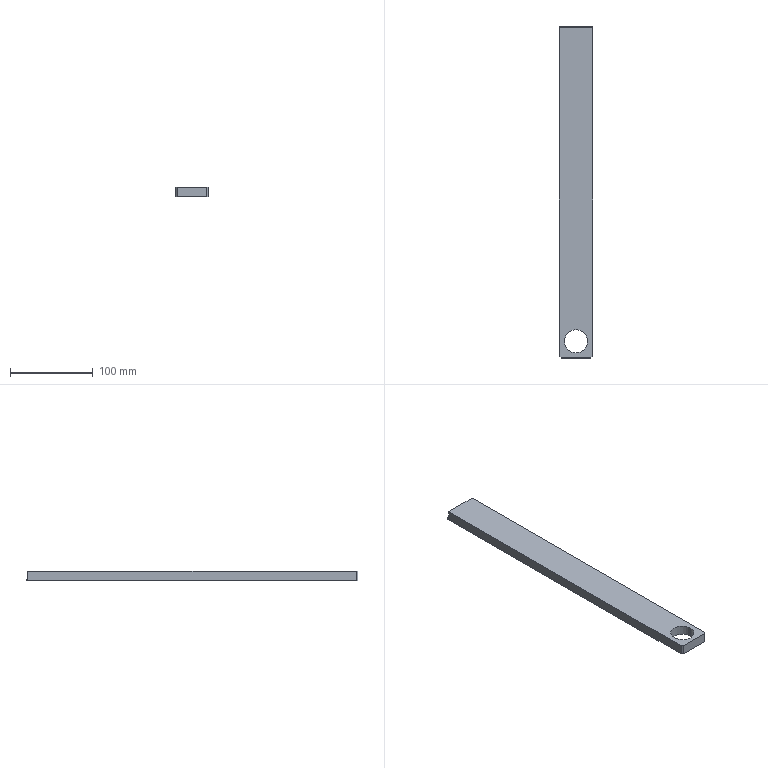Part | STEP file | 11-FG-B05811 | 1 solid | 28 faces | box 40 x 400 x 12 mm | volume 182663 mm3 | cylinder 10 | plane 10 | cone 8 | commonest cylinder face diameters 5 x8 28 x2
STEP:
#1=CARTESIAN_POINT('',(15.,386.,4.5));
#2=VERTEX_POINT('',#1);
#3=CARTESIAN_POINT('',(15.,386.,9.5));
#4=VERTEX_POINT('',#3);
#5=CARTESIAN_POINT('',(15.,386.,7.));
#6=DIRECTION('',(0.,1.,0.));
#7=DIRECTION('',(0.,0.,1.));
#8=AXIS2_PLACEMENT_3D('',#5,#6,#7);
#9=CIRCLE('',#8,2.5);
#10=EDGE_CURVE('',#2,#4,#9,.T.);
#11=ORIENTED_EDGE('',*,*,#10,.F.);
#12=CARTESIAN_POINT('',(15.,398.,4.5));
#13=VERTEX_POINT('',#12);
#14=CARTESIAN_POINT('',(15.,398.,4.5));
#15=DIRECTION('',(0.,1.,0.));
#16=VECTOR('',#15,1000.);
#17=LINE('',#14,#16);
#18=EDGE_CURVE('',#2,#13,#17,.T.);
#19=ORIENTED_EDGE('',*,*,#18,.T.);
#20=CARTESIAN_POINT('',(15.,398.,9.5));
#21=VERTEX_POINT('',#20);
#22=CARTESIAN_POINT('',(15.,398.,7.));
#23=DIRECTION('',(0.,1.,0.));
#24=DIRECTION('',(0.,0.,1.));
#25=AXIS2_PLACEMENT_3D('',#22,#23,#24);
#26=CIRCLE('',#25,2.5);
#27=EDGE_CURVE('',#13,#21,#26,.T.);
#28=ORIENTED_EDGE('',*,*,#27,.T.);
#29=CARTESIAN_POINT('',(15.,398.,9.5));
#30=DIRECTION('',(0.,1.,0.));
#31=VECTOR('',#30,1000.);
#32=LINE('',#29,#31);
#33=EDGE_CURVE('',#4,#21,#32,.T.);
#34=ORIENTED_EDGE('',*,*,#33,.F.);
#35=EDGE_LOOP('',(#11,#19,#28,#34));
#36=FACE_OUTER_BOUND('',#35,.T.);
#37=CARTESIAN_POINT('',(15.,398.,7.));
#38=DIRECTION('',(0.,1.,0.));
#39=DIRECTION('',(0.,0.,1.));
#40=AXIS2_PLACEMENT_3D('',#37,#38,#39);
#41=CYLINDRICAL_SURFACE('',#40,2.5);
#42=ADVANCED_FACE('',(#36),#41,.F.);
#43=CARTESIAN_POINT('',(15.,384.498,7.));
#44=VERTEX_POINT('',#43);
#45=CARTESIAN_POINT('',(15.,386.,9.5));
#46=DIRECTION('',(0.,0.515,0.8572));
#47=VECTOR('',#46,1000.);
#48=LINE('',#45,#47);
#49=EDGE_CURVE('',#44,#4,#48,.T.);
#50=ORIENTED_EDGE('',*,*,#49,.F.);
#51=CARTESIAN_POINT('',(15.,386.,4.5));
#52=DIRECTION('',(0.,0.515,-0.8572));
#53=VECTOR('',#52,1000.);
#54=LINE('',#51,#53);
#55=EDGE_CURVE('',#44,#2,#54,.T.);
#56=ORIENTED_EDGE('',*,*,#55,.T.);
#57=ORIENTED_EDGE('',*,*,#10,.T.);
#58=EDGE_LOOP('',(#50,#56,#57));
#59=FACE_OUTER_BOUND('',#58,.T.);
#60=CARTESIAN_POINT('',(15.,386.,7.));
#61=DIRECTION('',(0.,1.,0.));
#62=DIRECTION('',(0.,0.,1.));
#63=AXIS2_PLACEMENT_3D('',#60,#61,#62);
#64=CONICAL_SURFACE('',#63,2.5,1.03);
#65=ADVANCED_FACE('',(#59),#64,.F.);
#66=CARTESIAN_POINT('',(25.,386.,4.5));
#67=VERTEX_POINT('',#66);
#68=CARTESIAN_POINT('',(25.,386.,9.5));
#69=VERTEX_POINT('',#68);
#70=CARTESIAN_POINT('',(25.,386.,7.));
#71=DIRECTION('',(0.,1.,0.));
#72=DIRECTION('',(0.,0.,1.));
#73=AXIS2_PLACEMENT_3D('',#70,#71,#72);
#74=CIRCLE('',#73,2.5);
#75=EDGE_CURVE('',#67,#69,#74,.T.);
#76=ORIENTED_EDGE('',*,*,#75,.F.);
#77=CARTESIAN_POINT('',(25.,398.,4.5));
#78=VERTEX_POINT('',#77);
#79=CARTESIAN_POINT('',(25.,398.,4.5));
#80=DIRECTION('',(0.,1.,0.));
#81=VECTOR('',#80,1000.);
#82=LINE('',#79,#81);
#83=EDGE_CURVE('',#67,#78,#82,.T.);
#84=ORIENTED_EDGE('',*,*,#83,.T.);
#85=CARTESIAN_POINT('',(25.,398.,9.5));
#86=VERTEX_POINT('',#85);
#87=CARTESIAN_POINT('',(25.,398.,7.));
#88=DIRECTION('',(0.,1.,0.));
#89=DIRECTION('',(0.,0.,1.));
#90=AXIS2_PLACEMENT_3D('',#87,#88,#89);
#91=CIRCLE('',#90,2.5);
#92=EDGE_CURVE('',#78,#86,#91,.T.);
#93=ORIENTED_EDGE('',*,*,#92,.T.);
#94=CARTESIAN_POINT('',(25.,398.,9.5));
#95=DIRECTION('',(0.,1.,0.));
#96=VECTOR('',#95,1000.);
#97=LINE('',#94,#96);
#98=EDGE_CURVE('',#69,#86,#97,.T.);
#99=ORIENTED_EDGE('',*,*,#98,.F.);
#100=EDGE_LOOP('',(#76,#84,#93,#99));
#101=FACE_OUTER_BOUND('',#100,.T.);
#102=CARTESIAN_POINT('',(25.,398.,7.));
#103=DIRECTION('',(0.,1.,0.));
#104=DIRECTION('',(0.,0.,1.));
#105=AXIS2_PLACEMENT_3D('',#102,#103,#104);
#106=CYLINDRICAL_SURFACE('',#105,2.5);
#107=ADVANCED_FACE('',(#101),#106,.F.);
#108=CARTESIAN_POINT('',(25.,384.498,7.));
#109=VERTEX_POINT('',#108);
#110=CARTESIAN_POINT('',(25.,386.,9.5));
#111=DIRECTION('',(0.,0.515,0.8572));
#112=VECTOR('',#111,1000.);
#113=LINE('',#110,#112);
#114=EDGE_CURVE('',#109,#69,#113,.T.);
#115=ORIENTED_EDGE('',*,*,#114,.F.);
#116=CARTESIAN_POINT('',(25.,386.,4.5));
#117=DIRECTION('',(0.,0.515,-0.8572));
#118=VECTOR('',#117,1000.);
#119=LINE('',#116,#118);
#120=EDGE_CURVE('',#109,#67,#119,.T.);
#121=ORIENTED_EDGE('',*,*,#120,.T.);
#122=ORIENTED_EDGE('',*,*,#75,.T.);
#123=EDGE_LOOP('',(#115,#121,#122));
#124=FACE_OUTER_BOUND('',#123,.T.);
#125=CARTESIAN_POINT('',(25.,386.,7.));
#126=DIRECTION('',(0.,1.,0.));
#127=DIRECTION('',(0.,0.,1.));
#128=AXIS2_PLACEMENT_3D('',#125,#126,#127);
#129=CONICAL_SURFACE('',#128,2.5,1.03);
#130=ADVANCED_FACE('',(#124),#129,.F.);
#131=CARTESIAN_POINT('',(7.,383.,4.5));
#132=VERTEX_POINT('',#131);
#133=CARTESIAN_POINT('',(7.,383.,9.5));
#134=VERTEX_POINT('',#133);
#135=CARTESIAN_POINT('',(7.,383.,7.));
#136=DIRECTION('',(0.,1.,0.));
#137=DIRECTION('',(0.,0.,1.));
#138=AXIS2_PLACEMENT_3D('',#135,#136,#137);
#139=CIRCLE('',#138,2.5);
#140=EDGE_CURVE('',#132,#134,#139,.T.);
#141=ORIENTED_EDGE('',*,*,#140,.F.);
#142=CARTESIAN_POINT('',(7.,398.,4.5));
#143=VERTEX_POINT('',#142);
#144=CARTESIAN_POINT('',(7.,398.,4.5));
#145=DIRECTION('',(0.,1.,0.));
#146=VECTOR('',#145,1000.);
#147=LINE('',#144,#146);
#148=EDGE_CURVE('',#132,#143,#147,.T.);
#149=ORIENTED_EDGE('',*,*,#148,.T.);
#150=CARTESIAN_POINT('',(7.,398.,9.5));
#151=VERTEX_POINT('',#150);
#152=CARTESIAN_POINT('',(7.,398.,7.));
#153=DIRECTION('',(0.,1.,0.));
#154=DIRECTION('',(0.,0.,1.));
#155=AXIS2_PLACEMENT_3D('',#152,#153,#154);
#156=CIRCLE('',#155,2.5);
#157=EDGE_CURVE('',#143,#151,#156,.T.);
#158=ORIENTED_EDGE('',*,*,#157,.T.);
#159=CARTESIAN_POINT('',(7.,398.,9.5));
#160=DIRECTION('',(0.,1.,0.));
#161=VECTOR('',#160,1000.);
#162=LINE('',#159,#161);
#163=EDGE_CURVE('',#134,#151,#162,.T.);
#164=ORIENTED_EDGE('',*,*,#163,.F.);
#165=EDGE_LOOP('',(#141,#149,#158,#164));
#166=FACE_OUTER_BOUND('',#165,.T.);
#167=CARTESIAN_POINT('',(7.,398.,7.));
#168=DIRECTION('',(0.,1.,0.));
#169=DIRECTION('',(0.,0.,1.));
#170=AXIS2_PLACEMENT_3D('',#167,#168,#169);
#171=CYLINDRICAL_SURFACE('',#170,2.5);
#172=ADVANCED_FACE('',(#166),#171,.F.);
#173=CARTESIAN_POINT('',(7.,381.498,7.));
#174=VERTEX_POINT('',#173);
#175=CARTESIAN_POINT('',(7.,383.,9.5));
#176=DIRECTION('',(0.,0.515,0.8572));
#177=VECTOR('',#176,1000.);
#178=LINE('',#175,#177);
#179=EDGE_CURVE('',#174,#134,#178,.T.);
#180=ORIENTED_EDGE('',*,*,#179,.F.);
#181=CARTESIAN_POINT('',(7.,383.,4.5));
#182=DIRECTION('',(0.,0.515,-0.8572));
#183=VECTOR('',#182,1000.);
#184=LINE('',#181,#183);
#185=EDGE_CURVE('',#174,#132,#184,.T.);
#186=ORIENTED_EDGE('',*,*,#185,.T.);
#187=ORIENTED_EDGE('',*,*,#140,.T.);
#188=EDGE_LOOP('',(#180,#186,#187));
#189=FACE_OUTER_BOUND('',#188,.T.);
#190=CARTESIAN_POINT('',(7.,383.,7.));
#191=DIRECTION('',(0.,1.,0.));
#192=DIRECTION('',(0.,0.,1.));
#193=AXIS2_PLACEMENT_3D('',#190,#191,#192);
#194=CONICAL_SURFACE('',#193,2.5,1.03);
#195=ADVANCED_FACE('',(#189),#194,.F.);
#196=CARTESIAN_POINT('',(33.,383.,4.5));
#197=VERTEX_POINT('',#196);
#198=CARTESIAN_POINT('',(33.,383.,9.5));
#199=VERTEX_POINT('',#198);
#200=CARTESIAN_POINT('',(33.,383.,7.));
#201=DIRECTION('',(0.,1.,0.));
#202=DIRECTION('',(0.,0.,1.));
#203=AXIS2_PLACEMENT_3D('',#200,#201,#202);
#204=CIRCLE('',#203,2.5);
#205=EDGE_CURVE('',#197,#199,#204,.T.);
#206=ORIENTED_EDGE('',*,*,#205,.F.);
#207=CARTESIAN_POINT('',(33.,398.,4.5));
#208=VERTEX_POINT('',#207);
#209=CARTESIAN_POINT('',(33.,398.,4.5));
#210=DIRECTION('',(0.,1.,0.));
#211=VECTOR('',#210,1000.);
#212=LINE('',#209,#211);
#213=EDGE_CURVE('',#197,#208,#212,.T.);
#214=ORIENTED_EDGE('',*,*,#213,.T.);
#215=CARTESIAN_POINT('',(33.,398.,9.5));
#216=VERTEX_POINT('',#215);
#217=CARTESIAN_POINT('',(33.,398.,7.));
#218=DIRECTION('',(0.,1.,0.));
#219=DIRECTION('',(0.,0.,1.));
#220=AXIS2_PLACEMENT_3D('',#217,#218,#219);
#221=CIRCLE('',#220,2.5);
#222=EDGE_CURVE('',#208,#216,#221,.T.);
#223=ORIENTED_EDGE('',*,*,#222,.T.);
#224=CARTESIAN_POINT('',(33.,398.,9.5));
#225=DIRECTION('',(0.,1.,0.));
#226=VECTOR('',#225,1000.);
#227=LINE('',#224,#226);
#228=EDGE_CURVE('',#199,#216,#227,.T.);
#229=ORIENTED_EDGE('',*,*,#228,.F.);
#230=EDGE_LOOP('',(#206,#214,#223,#229));
#231=FACE_OUTER_BOUND('',#230,.T.);
#232=CARTESIAN_POINT('',(33.,398.,7.));
#233=DIRECTION('',(0.,1.,0.));
#234=DIRECTION('',(0.,0.,1.));
#235=AXIS2_PLACEMENT_3D('',#232,#233,#234);
#236=CYLINDRICAL_SURFACE('',#235,2.5);
#237=ADVANCED_FACE('',(#231),#236,.F.);
#238=CARTESIAN_POINT('',(33.,381.498,7.));
#239=VERTEX_POINT('',#238);
#240=CARTESIAN_POINT('',(33.,383.,9.5));
#241=DIRECTION('',(0.,0.515,0.8572));
#242=VECTOR('',#241,1000.);
#243=LINE('',#240,#242);
#244=EDGE_CURVE('',#239,#199,#243,.T.);
#245=ORIENTED_EDGE('',*,*,#244,.F.);
#246=CARTESIAN_POINT('',(33.,383.,4.5));
#247=DIRECTION('',(0.,0.515,-0.8572));
#248=VECTOR('',#247,1000.);
#249=LINE('',#246,#248);
#250=EDGE_CURVE('',#239,#197,#249,.T.);
#251=ORIENTED_EDGE('',*,*,#250,.T.);
#252=ORIENTED_EDGE('',*,*,#205,.T.);
#253=EDGE_LOOP('',(#245,#251,#252));
#254=FACE_OUTER_BOUND('',#253,.T.);
#255=CARTESIAN_POINT('',(33.,383.,7.));
#256=DIRECTION('',(0.,1.,0.));
#257=DIRECTION('',(0.,0.,1.));
#258=AXIS2_PLACEMENT_3D('',#255,#256,#257);
#259=CONICAL_SURFACE('',#258,2.5,1.03);
#260=ADVANCED_FACE('',(#254),#259,.F.);
#261=CARTESIAN_POINT('',(6.,20.,0.));
#262=VERTEX_POINT('',#261);
#263=CARTESIAN_POINT('',(34.,20.,0.));
#264=VERTEX_POINT('',#263);
#265=CARTESIAN_POINT('',(20.,20.,0.));
#266=DIRECTION('',(0.,0.,1.));
#267=DIRECTION('',(1.,0.,0.));
#268=AXIS2_PLACEMENT_3D('',#265,#266,#267);
#269=CIRCLE('',#268,14.);
#270=EDGE_CURVE('',#262,#264,#269,.T.);
#271=ORIENTED_EDGE('',*,*,#270,.F.);
#272=CARTESIAN_POINT('',(6.,20.,12.));
#273=VERTEX_POINT('',#272);
#274=CARTESIAN_POINT('',(6.,20.,0.));
#275=DIRECTION('',(0.,0.,1.));
#276=VECTOR('',#275,1000.);
#277=LINE('',#274,#276);
#278=EDGE_CURVE('',#262,#273,#277,.T.);
#279=ORIENTED_EDGE('',*,*,#278,.T.);
#280=CARTESIAN_POINT('',(34.,20.,12.));
#281=VERTEX_POINT('',#280);
#282=CARTESIAN_POINT('',(20.,20.,12.));
#283=DIRECTION('',(0.,0.,1.));
#284=DIRECTION('',(1.,0.,0.));
#285=AXIS2_PLACEMENT_3D('',#282,#283,#284);
#286=CIRCLE('',#285,14.);
#287=EDGE_CURVE('',#273,#281,#286,.T.);
#288=ORIENTED_EDGE('',*,*,#287,.T.);
#289=CARTESIAN_POINT('',(34.,20.,0.));
#290=DIRECTION('',(0.,0.,1.));
#291=VECTOR('',#290,1000.);
#292=LINE('',#289,#291);
#293=EDGE_CURVE('',#264,#281,#292,.T.);
#294=ORIENTED_EDGE('',*,*,#293,.F.);
#295=EDGE_LOOP('',(#271,#279,#288,#294));
#296=FACE_OUTER_BOUND('',#295,.T.);
#297=CARTESIAN_POINT('',(20.,20.,0.));
#298=DIRECTION('',(0.,0.,1.));
#299=DIRECTION('',(1.,0.,0.));
#300=AXIS2_PLACEMENT_3D('',#297,#298,#299);
#301=CYLINDRICAL_SURFACE('',#300,14.);
#302=ADVANCED_FACE('',(#296),#301,.F.);
#303=CARTESIAN_POINT('',(0.,398.,12.));
#304=VERTEX_POINT('',#303);
#305=CARTESIAN_POINT('',(0.,2.,12.));
#306=VERTEX_POINT('',#305);
#307=CARTESIAN_POINT('',(0.,0.,12.));
#308=DIRECTION('',(0.,-1.,0.));
#309=VECTOR('',#308,1000.);
#310=LINE('',#307,#309);
#311=EDGE_CURVE('',#304,#306,#310,.T.);
#312=ORIENTED_EDGE('',*,*,#311,.F.);
#313=CARTESIAN_POINT('',(0.,398.,2.));
#314=VERTEX_POINT('',#313);
#315=CARTESIAN_POINT('',(0.,398.,12.));
#316=DIRECTION('',(0.,0.,1.));
#317=VECTOR('',#316,1000.);
#318=LINE('',#315,#317);
#319=EDGE_CURVE('',#314,#304,#318,.T.);
#320=ORIENTED_EDGE('',*,*,#319,.F.);
#321=CARTESIAN_POINT('',(0.,400.,2.));
#322=VERTEX_POINT('',#321);
#323=CARTESIAN_POINT('',(0.,400.,2.));
#324=DIRECTION('',(0.,-1.,0.));
#325=VECTOR('',#324,1000.);
#326=LINE('',#323,#325);
#327=EDGE_CURVE('',#322,#314,#326,.T.);
#328=ORIENTED_EDGE('',*,*,#327,.F.);
#329=CARTESIAN_POINT('',(0.,400.,0.));
#330=VERTEX_POINT('',#329);
#331=CARTESIAN_POINT('',(0.,400.,12.));
#332=DIRECTION('',(0.,0.,-1.));
#333=VECTOR('',#332,1000.);
#334=LINE('',#331,#333);
#335=EDGE_CURVE('',#322,#330,#334,.T.);
#336=ORIENTED_EDGE('',*,*,#335,.T.);
#337=CARTESIAN_POINT('',(0.,2.,0.));
#338=VERTEX_POINT('',#337);
#339=CARTESIAN_POINT('',(0.,0.,0.));
#340=DIRECTION('',(0.,-1.,0.));
#341=VECTOR('',#340,1000.);
#342=LINE('',#339,#341);
#343=EDGE_CURVE('',#330,#338,#342,.T.);
#344=ORIENTED_EDGE('',*,*,#343,.T.);
#345=CARTESIAN_POINT('',(0.,2.,12.));
#346=DIRECTION('',(0.,0.,1.));
#347=VECTOR('',#346,1000.);
#348=LINE('',#345,#347);
#349=EDGE_CURVE('',#338,#306,#348,.T.);
#350=ORIENTED_EDGE('',*,*,#349,.T.);
#351=EDGE_LOOP('',(#312,#320,#328,#336,#344,#350));
#352=FACE_OUTER_BOUND('',#351,.T.);
#353=CARTESIAN_POINT('',(0.,0.,12.));
#354=DIRECTION('',(1.,0.,0.));
#355=DIRECTION('',(0.,1.,0.));
#356=AXIS2_PLACEMENT_3D('',#353,#354,#355);
#357=PLANE('',#356);
#358=ADVANCED_FACE('',(#352),#357,.F.);
#359=CARTESIAN_POINT('',(2.,0.,0.));
#360=VERTEX_POINT('',#359);
#361=CARTESIAN_POINT('',(38.,0.,0.));
#362=VERTEX_POINT('',#361);
#363=CARTESIAN_POINT('',(0.,0.,0.));
#364=DIRECTION('',(1.,0.,0.));
#365=VECTOR('',#364,1000.);
#366=LINE('',#363,#365);
#367=EDGE_CURVE('',#360,#362,#366,.T.);
#368=ORIENTED_EDGE('',*,*,#367,.T.);
#369=CARTESIAN_POINT('',(38.,0.,12.));
#370=VERTEX_POINT('',#369);
#371=CARTESIAN_POINT('',(38.,0.,12.));
#372=DIRECTION('',(0.,0.,1.));
#373=VECTOR('',#372,1000.);
#374=LINE('',#371,#373);
#375=EDGE_CURVE('',#362,#370,#374,.T.);
#376=ORIENTED_EDGE('',*,*,#375,.T.);
#377=CARTESIAN_POINT('',(2.,0.,12.));
#378=VERTEX_POINT('',#377);
#379=CARTESIAN_POINT('',(0.,0.,12.));
#380=DIRECTION('',(1.,0.,0.));
#381=VECTOR('',#380,1000.);
#382=LINE('',#379,#381);
#383=EDGE_CURVE('',#378,#370,#382,.T.);
#384=ORIENTED_EDGE('',*,*,#383,.F.);
#385=CARTESIAN_POINT('',(2.,0.,12.));
#386=DIRECTION('',(0.,0.,-1.));
#387=VECTOR('',#386,1000.);
#388=LINE('',#385,#387);
#389=EDGE_CURVE('',#378,#360,#388,.T.);
#390=ORIENTED_EDGE('',*,*,#389,.T.);
#391=EDGE_LOOP('',(#368,#376,#384,#390));
#392=FACE_OUTER_BOUND('',#391,.T.);
#393=CARTESIAN_POINT('',(0.,0.,12.));
#394=DIRECTION('',(0.,1.,0.));
#395=DIRECTION('',(0.,0.,1.));
#396=AXIS2_PLACEMENT_3D('',#393,#394,#395);
#397=PLANE('',#396);
#398=ADVANCED_FACE('',(#392),#397,.F.);
#399=CARTESIAN_POINT('',(40.,400.,2.));
#400=VERTEX_POINT('',#399);
#401=CARTESIAN_POINT('',(40.,398.,2.));
#402=VERTEX_POINT('',#401);
#403=CARTESIAN_POINT('',(40.,0.,2.));
#404=DIRECTION('',(0.,-1.,0.));
#405=VECTOR('',#404,1000.);
#406=LINE('',#403,#405);
#407=EDGE_CURVE('',#400,#402,#406,.T.);
#408=ORIENTED_EDGE('',*,*,#407,.T.);
#409=CARTESIAN_POINT('',(40.,398.,12.));
#410=VERTEX_POINT('',#409);
#411=CARTESIAN_POINT('',(40.,398.,12.));
#412=DIRECTION('',(0.,0.,1.));
#413=VECTOR('',#412,1000.);
#414=LINE('',#411,#413);
#415=EDGE_CURVE('',#402,#410,#414,.T.);
#416=ORIENTED_EDGE('',*,*,#415,.T.);
#417=CARTESIAN_POINT('',(40.,2.,12.));
#418=VERTEX_POINT('',#417);
#419=CARTESIAN_POINT('',(40.,0.,12.));
#420=DIRECTION('',(0.,1.,0.));
#421=VECTOR('',#420,1000.);
#422=LINE('',#419,#421);
#423=EDGE_CURVE('',#418,#410,#422,.T.);
#424=ORIENTED_EDGE('',*,*,#423,.F.);
#425=CARTESIAN_POINT('',(40.,2.,0.));
#426=VERTEX_POINT('',#425);
#427=CARTESIAN_POINT('',(40.,2.,12.));
#428=DIRECTION('',(0.,0.,-1.));
#429=VECTOR('',#428,1000.);
#430=LINE('',#427,#429);
#431=EDGE_CURVE('',#418,#426,#430,.T.);
#432=ORIENTED_EDGE('',*,*,#431,.T.);
#433=CARTESIAN_POINT('',(40.,400.,0.));
#434=VERTEX_POINT('',#433);
#435=CARTESIAN_POINT('',(40.,0.,0.));
#436=DIRECTION('',(0.,1.,0.));
#437=VECTOR('',#436,1000.);
#438=LINE('',#435,#437);
#439=EDGE_CURVE('',#426,#434,#438,.T.);
#440=ORIENTED_EDGE('',*,*,#439,.T.);
#441=CARTESIAN_POINT('',(40.,400.,12.));
#442=DIRECTION('',(0.,0.,-1.));
#443=VECTOR('',#442,1000.);
#444=LINE('',#441,#443);
#445=EDGE_CURVE('',#400,#434,#444,.T.);
#446=ORIENTED_EDGE('',*,*,#445,.F.);
#447=EDGE_LOOP('',(#408,#416,#424,#432,#440,#446));
#448=FACE_OUTER_BOUND('',#447,.T.);
#449=CARTESIAN_POINT('',(40.,0.,12.));
#450=DIRECTION('',(-1.,0.,0.));
#451=DIRECTION('',(0.,-1.,0.));
#452=AXIS2_PLACEMENT_3D('',#449,#450,#451);
#453=PLANE('',#452);
#454=ADVANCED_FACE('',(#448),#453,.F.);
#455=ORIENTED_EDGE('',*,*,#335,.F.);
#456=CARTESIAN_POINT('',(59.,400.,2.));
#457=DIRECTION('',(-1.,0.,0.));
#458=VECTOR('',#457,1000.);
#459=LINE('',#456,#458);
#460=EDGE_CURVE('',#400,#322,#459,.T.);
#461=ORIENTED_EDGE('',*,*,#460,.F.);
#462=ORIENTED_EDGE('',*,*,#445,.T.);
#463=CARTESIAN_POINT('',(0.,400.,0.));
#464=DIRECTION('',(-1.,0.,0.));
#465=VECTOR('',#464,1000.);
#466=LINE('',#463,#465);
#467=EDGE_CURVE('',#434,#330,#466,.T.);
#468=ORIENTED_EDGE('',*,*,#467,.T.);
#469=EDGE_LOOP('',(#455,#461,#462,#468));
#470=FACE_OUTER_BOUND('',#469,.T.);
#471=CARTESIAN_POINT('',(0.,400.,12.));
#472=DIRECTION('',(0.,-1.,0.));
#473=DIRECTION('',(0.,0.,-1.));
#474=AXIS2_PLACEMENT_3D('',#471,#472,#473);
#475=PLANE('',#474);
#476=ADVANCED_FACE('',(#470),#475,.F.);
#477=CARTESIAN_POINT('',(20.,20.,12.));
#478=DIRECTION('',(0.,0.,1.));
#479=DIRECTION('',(1.,0.,0.));
#480=AXIS2_PLACEMENT_3D('',#477,#478,#479);
#481=CIRCLE('',#480,14.);
#482=EDGE_CURVE('',#281,#273,#481,.T.);
#483=ORIENTED_EDGE('',*,*,#482,.F.);
#484=ORIENTED_EDGE('',*,*,#287,.F.);
#485=EDGE_LOOP('',(#483,#484));
#486=FACE_BOUND('',#485,.T.);
#487=ORIENTED_EDGE('',*,*,#423,.T.);
#488=CARTESIAN_POINT('',(0.,398.,12.));
#489=DIRECTION('',(-1.,0.,0.));
#490=VECTOR('',#489,1000.);
#491=LINE('',#488,#490);
#492=EDGE_CURVE('',#410,#304,#491,.T.);
#493=ORIENTED_EDGE('',*,*,#492,.T.);
#494=ORIENTED_EDGE('',*,*,#311,.T.);
#495=CARTESIAN_POINT('',(2.,0.,12.));
#496=DIRECTION('',(0.7071,-0.7071,0.));
#497=VECTOR('',#496,1000.);
#498=LINE('',#495,#497);
#499=EDGE_CURVE('',#306,#378,#498,.T.);
#500=ORIENTED_EDGE('',*,*,#499,.T.);
#501=ORIENTED_EDGE('',*,*,#383,.T.);
#502=CARTESIAN_POINT('',(40.,2.,12.));
#503=DIRECTION('',(0.7071,0.7071,0.));
#504=VECTOR('',#503,1000.);
#505=LINE('',#502,#504);
#506=EDGE_CURVE('',#370,#418,#505,.T.);
#507=ORIENTED_EDGE('',*,*,#506,.T.);
#508=EDGE_LOOP('',(#487,#493,#494,#500,#501,#507));
#509=FACE_OUTER_BOUND('',#508,.T.);
#510=CARTESIAN_POINT('',(0.,400.,12.));
#511=DIRECTION('',(0.,0.,-1.));
#512=DIRECTION('',(-1.,0.,0.));
#513=AXIS2_PLACEMENT_3D('',#510,#511,#512);
#514=PLANE('',#513);
#515=ADVANCED_FACE('',(#486,#509),#514,.F.);
#516=CARTESIAN_POINT('',(20.,20.,0.));
#517=DIRECTION('',(0.,0.,1.));
#518=DIRECTION('',(1.,0.,0.));
#519=AXIS2_PLACEMENT_3D('',#516,#517,#518);
#520=CIRCLE('',#519,14.);
#521=EDGE_CURVE('',#264,#262,#520,.T.);
#522=ORIENTED_EDGE('',*,*,#521,.T.);
#523=ORIENTED_EDGE('',*,*,#270,.T.);
#524=EDGE_LOOP('',(#522,#523));
#525=FACE_BOUND('',#524,.T.);
#526=ORIENTED_EDGE('',*,*,#439,.F.);
#527=CARTESIAN_POINT('',(219.,181.,0.));
#528=DIRECTION('',(-0.7071,-0.7071,0.));
#529=VECTOR('',#528,1000.);
#530=LINE('',#527,#529);
#531=EDGE_CURVE('',#426,#362,#530,.T.);
#532=ORIENTED_EDGE('',*,*,#531,.T.);
#533=ORIENTED_EDGE('',*,*,#367,.F.);
#534=CARTESIAN_POINT('',(-199.,201.,0.));
#535=DIRECTION('',(-0.7071,0.7071,0.));
#536=VECTOR('',#535,1000.);
#537=LINE('',#534,#536);
#538=EDGE_CURVE('',#360,#338,#537,.T.);
#539=ORIENTED_EDGE('',*,*,#538,.T.);
#540=ORIENTED_EDGE('',*,*,#343,.F.);
#541=ORIENTED_EDGE('',*,*,#467,.F.);
#542=EDGE_LOOP('',(#526,#532,#533,#539,#540,#541));
#543=FACE_OUTER_BOUND('',#542,.T.);
#544=CARTESIAN_POINT('',(0.,400.,0.));
#545=DIRECTION('',(0.,0.,-1.));
#546=DIRECTION('',(-1.,0.,0.));
#547=AXIS2_PLACEMENT_3D('',#544,#545,#546);
#548=PLANE('',#547);
#549=ADVANCED_FACE('',(#525,#543),#548,.T.);
#550=ORIENTED_EDGE('',*,*,#278,.F.);
#551=ORIENTED_EDGE('',*,*,#521,.F.);
#552=ORIENTED_EDGE('',*,*,#293,.T.);
#553=ORIENTED_EDGE('',*,*,#482,.T.);
#554=EDGE_LOOP('',(#550,#551,#552,#553));
#555=FACE_OUTER_BOUND('',#554,.T.);
#556=CARTESIAN_POINT('',(20.,20.,0.));
#557=DIRECTION('',(0.,0.,1.));
#558=DIRECTION('',(1.,0.,0.));
#559=AXIS2_PLACEMENT_3D('',#556,#557,#558);
#560=CYLINDRICAL_SURFACE('',#559,14.);
#561=ADVANCED_FACE('',(#555),#560,.F.);
#562=ORIENTED_EDGE('',*,*,#506,.F.);
#563=ORIENTED_EDGE('',*,*,#375,.F.);
#564=ORIENTED_EDGE('',*,*,#531,.F.);
#565=ORIENTED_EDGE('',*,*,#431,.F.);
#566=EDGE_LOOP('',(#562,#563,#564,#565));
#567=FACE_OUTER_BOUND('',#566,.T.);
#568=CARTESIAN_POINT('',(40.,2.,12.));
#569=DIRECTION('',(-0.7071,0.7071,0.));
#570=DIRECTION('',(-0.7071,-0.7071,0.));
#571=AXIS2_PLACEMENT_3D('',#568,#569,#570);
#572=PLANE('',#571);
#573=ADVANCED_FACE('',(#567),#572,.F.);
#574=ORIENTED_EDGE('',*,*,#499,.F.);
#575=ORIENTED_EDGE('',*,*,#349,.F.);
#576=ORIENTED_EDGE('',*,*,#538,.F.);
#577=ORIENTED_EDGE('',*,*,#389,.F.);
#578=EDGE_LOOP('',(#574,#575,#576,#577));
#579=FACE_OUTER_BOUND('',#578,.T.);
#580=CARTESIAN_POINT('',(2.,0.,12.));
#581=DIRECTION('',(0.7071,0.7071,0.));
#582=DIRECTION('',(-0.7071,0.7071,0.));
#583=AXIS2_PLACEMENT_3D('',#580,#581,#582);
#584=PLANE('',#583);
#585=ADVANCED_FACE('',(#579),#584,.F.);
#586=ORIENTED_EDGE('',*,*,#460,.T.);
#587=ORIENTED_EDGE('',*,*,#327,.T.);
#588=CARTESIAN_POINT('',(59.,398.,2.));
#589=DIRECTION('',(-1.,0.,0.));
#590=VECTOR('',#589,1000.);
#591=LINE('',#588,#590);
#592=EDGE_CURVE('',#402,#314,#591,.T.);
#593=ORIENTED_EDGE('',*,*,#592,.F.);
#594=ORIENTED_EDGE('',*,*,#407,.F.);
#595=EDGE_LOOP('',(#586,#587,#593,#594));
#596=FACE_OUTER_BOUND('',#595,.T.);
#597=CARTESIAN_POINT('',(59.,400.,2.));
#598=DIRECTION('',(0.,0.,-1.));
#599=DIRECTION('',(-1.,0.,0.));
#600=AXIS2_PLACEMENT_3D('',#597,#598,#599);
#601=PLANE('',#600);
#602=ADVANCED_FACE('',(#596),#601,.F.);
#603=CARTESIAN_POINT('',(15.,398.,7.));
#604=DIRECTION('',(0.,1.,0.));
#605=DIRECTION('',(0.,0.,1.));
#606=AXIS2_PLACEMENT_3D('',#603,#604,#605);
#607=CIRCLE('',#606,2.5);
#608=EDGE_CURVE('',#21,#13,#607,.T.);
#609=ORIENTED_EDGE('',*,*,#608,.F.);
#610=ORIENTED_EDGE('',*,*,#27,.F.);
#611=EDGE_LOOP('',(#609,#610));
#612=FACE_BOUND('',#611,.T.);
#613=CARTESIAN_POINT('',(25.,398.,7.));
#614=DIRECTION('',(0.,1.,0.));
#615=DIRECTION('',(0.,0.,1.));
#616=AXIS2_PLACEMENT_3D('',#613,#614,#615);
#617=CIRCLE('',#616,2.5);
#618=EDGE_CURVE('',#86,#78,#617,.T.);
#619=ORIENTED_EDGE('',*,*,#618,.F.);
#620=ORIENTED_EDGE('',*,*,#92,.F.);
#621=EDGE_LOOP('',(#619,#620));
#622=FACE_BOUND('',#621,.T.);
#623=CARTESIAN_POINT('',(7.,398.,7.));
#624=DIRECTION('',(0.,1.,0.));
#625=DIRECTION('',(0.,0.,1.));
#626=AXIS2_PLACEMENT_3D('',#623,#624,#625);
#627=CIRCLE('',#626,2.5);
#628=EDGE_CURVE('',#151,#143,#627,.T.);
#629=ORIENTED_EDGE('',*,*,#628,.F.);
#630=ORIENTED_EDGE('',*,*,#157,.F.);
#631=EDGE_LOOP('',(#629,#630));
#632=FACE_BOUND('',#631,.T.);
#633=CARTESIAN_POINT('',(33.,398.,7.));
#634=DIRECTION('',(0.,1.,0.));
#635=DIRECTION('',(0.,0.,1.));
#636=AXIS2_PLACEMENT_3D('',#633,#634,#635);
#637=CIRCLE('',#636,2.5);
#638=EDGE_CURVE('',#216,#208,#637,.T.);
#639=ORIENTED_EDGE('',*,*,#638,.F.);
#640=ORIENTED_EDGE('',*,*,#222,.F.);
#641=EDGE_LOOP('',(#639,#640));
#642=FACE_BOUND('',#641,.T.);
#643=ORIENTED_EDGE('',*,*,#592,.T.);
#644=ORIENTED_EDGE('',*,*,#319,.T.);
#645=ORIENTED_EDGE('',*,*,#492,.F.);
#646=ORIENTED_EDGE('',*,*,#415,.F.);
#647=EDGE_LOOP('',(#643,#644,#645,#646));
#648=FACE_OUTER_BOUND('',#647,.T.);
#649=CARTESIAN_POINT('',(59.,398.,12.));
#650=DIRECTION('',(0.,-1.,0.));
#651=DIRECTION('',(1.,0.,0.));
#652=AXIS2_PLACEMENT_3D('',#649,#650,#651);
#653=PLANE('',#652);
#654=ADVANCED_FACE('',(#612,#622,#632,#642,#648),#653,.F.);
#655=ORIENTED_EDGE('',*,*,#250,.F.);
#656=ORIENTED_EDGE('',*,*,#244,.T.);
#657=CARTESIAN_POINT('',(33.,383.,7.));
#658=DIRECTION('',(0.,1.,0.));
#659=DIRECTION('',(0.,0.,1.));
#660=AXIS2_PLACEMENT_3D('',#657,#658,#659);
#661=CIRCLE('',#660,2.5);
#662=EDGE_CURVE('',#199,#197,#661,.T.);
#663=ORIENTED_EDGE('',*,*,#662,.T.);
#664=EDGE_LOOP('',(#655,#656,#663));
#665=FACE_OUTER_BOUND('',#664,.T.);
#666=CARTESIAN_POINT('',(33.,383.,7.));
#667=DIRECTION('',(0.,1.,0.));
#668=DIRECTION('',(0.,0.,1.));
#669=AXIS2_PLACEMENT_3D('',#666,#667,#668);
#670=CONICAL_SURFACE('',#669,2.5,1.03);
#671=ADVANCED_FACE('',(#665),#670,.F.);
#672=ORIENTED_EDGE('',*,*,#213,.F.);
#673=ORIENTED_EDGE('',*,*,#662,.F.);
#674=ORIENTED_EDGE('',*,*,#228,.T.);
#675=ORIENTED_EDGE('',*,*,#638,.T.);
#676=EDGE_LOOP('',(#672,#673,#674,#675));
#677=FACE_OUTER_BOUND('',#676,.T.);
#678=CARTESIAN_POINT('',(33.,398.,7.));
#679=DIRECTION('',(0.,1.,0.));
#680=DIRECTION('',(0.,0.,1.));
#681=AXIS2_PLACEMENT_3D('',#678,#679,#680);
#682=CYLINDRICAL_SURFACE('',#681,2.5);
#683=ADVANCED_FACE('',(#677),#682,.F.);
#684=ORIENTED_EDGE('',*,*,#185,.F.);
#685=ORIENTED_EDGE('',*,*,#179,.T.);
#686=CARTESIAN_POINT('',(7.,383.,7.));
#687=DIRECTION('',(0.,1.,0.));
#688=DIRECTION('',(0.,0.,1.));
#689=AXIS2_PLACEMENT_3D('',#686,#687,#688);
#690=CIRCLE('',#689,2.5);
#691=EDGE_CURVE('',#134,#132,#690,.T.);
#692=ORIENTED_EDGE('',*,*,#691,.T.);
#693=EDGE_LOOP('',(#684,#685,#692));
#694=FACE_OUTER_BOUND('',#693,.T.);
#695=CARTESIAN_POINT('',(7.,383.,7.));
#696=DIRECTION('',(0.,1.,0.));
#697=DIRECTION('',(0.,0.,1.));
#698=AXIS2_PLACEMENT_3D('',#695,#696,#697);
#699=CONICAL_SURFACE('',#698,2.5,1.03);
#700=ADVANCED_FACE('',(#694),#699,.F.);
#701=ORIENTED_EDGE('',*,*,#148,.F.);
#702=ORIENTED_EDGE('',*,*,#691,.F.);
#703=ORIENTED_EDGE('',*,*,#163,.T.);
#704=ORIENTED_EDGE('',*,*,#628,.T.);
#705=EDGE_LOOP('',(#701,#702,#703,#704));
#706=FACE_OUTER_BOUND('',#705,.T.);
#707=CARTESIAN_POINT('',(7.,398.,7.));
#708=DIRECTION('',(0.,1.,0.));
#709=DIRECTION('',(0.,0.,1.));
#710=AXIS2_PLACEMENT_3D('',#707,#708,#709);
#711=CYLINDRICAL_SURFACE('',#710,2.5);
#712=ADVANCED_FACE('',(#706),#711,.F.);
#713=ORIENTED_EDGE('',*,*,#120,.F.);
#714=ORIENTED_EDGE('',*,*,#114,.T.);
#715=CARTESIAN_POINT('',(25.,386.,7.));
#716=DIRECTION('',(0.,1.,0.));
#717=DIRECTION('',(0.,0.,1.));
#718=AXIS2_PLACEMENT_3D('',#715,#716,#717);
#719=CIRCLE('',#718,2.5);
#720=EDGE_CURVE('',#69,#67,#719,.T.);
#721=ORIENTED_EDGE('',*,*,#720,.T.);
#722=EDGE_LOOP('',(#713,#714,#721));
#723=FACE_OUTER_BOUND('',#722,.T.);
#724=CARTESIAN_POINT('',(25.,386.,7.));
#725=DIRECTION('',(0.,1.,0.));
#726=DIRECTION('',(0.,0.,1.));
#727=AXIS2_PLACEMENT_3D('',#724,#725,#726);
#728=CONICAL_SURFACE('',#727,2.5,1.03);
#729=ADVANCED_FACE('',(#723),#728,.F.);
#730=ORIENTED_EDGE('',*,*,#83,.F.);
#731=ORIENTED_EDGE('',*,*,#720,.F.);
#732=ORIENTED_EDGE('',*,*,#98,.T.);
#733=ORIENTED_EDGE('',*,*,#618,.T.);
#734=EDGE_LOOP('',(#730,#731,#732,#733));
#735=FACE_OUTER_BOUND('',#734,.T.);
#736=CARTESIAN_POINT('',(25.,398.,7.));
#737=DIRECTION('',(0.,1.,0.));
#738=DIRECTION('',(0.,0.,1.));
#739=AXIS2_PLACEMENT_3D('',#736,#737,#738);
#740=CYLINDRICAL_SURFACE('',#739,2.5);
#741=ADVANCED_FACE('',(#735),#740,.F.);
#742=ORIENTED_EDGE('',*,*,#55,.F.);
#743=ORIENTED_EDGE('',*,*,#49,.T.);
#744=CARTESIAN_POINT('',(15.,386.,7.));
#745=DIRECTION('',(0.,1.,0.));
#746=DIRECTION('',(0.,0.,1.));
#747=AXIS2_PLACEMENT_3D('',#744,#745,#746);
#748=CIRCLE('',#747,2.5);
#749=EDGE_CURVE('',#4,#2,#748,.T.);
#750=ORIENTED_EDGE('',*,*,#749,.T.);
#751=EDGE_LOOP('',(#742,#743,#750));
#752=FACE_OUTER_BOUND('',#751,.T.);
#753=CARTESIAN_POINT('',(15.,386.,7.));
#754=DIRECTION('',(0.,1.,0.));
#755=DIRECTION('',(0.,0.,1.));
#756=AXIS2_PLACEMENT_3D('',#753,#754,#755);
#757=CONICAL_SURFACE('',#756,2.5,1.03);
#758=ADVANCED_FACE('',(#752),#757,.F.);
#759=ORIENTED_EDGE('',*,*,#18,.F.);
#760=ORIENTED_EDGE('',*,*,#749,.F.);
#761=ORIENTED_EDGE('',*,*,#33,.T.);
#762=ORIENTED_EDGE('',*,*,#608,.T.);
#763=EDGE_LOOP('',(#759,#760,#761,#762));
#764=FACE_OUTER_BOUND('',#763,.T.);
#765=CARTESIAN_POINT('',(15.,398.,7.));
#766=DIRECTION('',(0.,1.,0.));
#767=DIRECTION('',(0.,0.,1.));
#768=AXIS2_PLACEMENT_3D('',#765,#766,#767);
#769=CYLINDRICAL_SURFACE('',#768,2.5);
#770=ADVANCED_FACE('',(#764),#769,.F.);
#771=CLOSED_SHELL('',(#42,#65,#107,#130,#172,#195,#237,#260,#302,#358,#398,#454,#476,#515,#549,#561,#573,#585,#602,#654,#671,#683,#700,#712,#729,#741,#758,#770));
#772=MANIFOLD_SOLID_BREP('',#771);
#773=CARTESIAN_POINT('',(0.,0.,0.));
#774=DIRECTION('',(0.,0.,1.));
#775=DIRECTION('',(1.,0.,0.));
#776=AXIS2_PLACEMENT_3D('',#773,#774,#775);
#777=(LENGTH_UNIT()NAMED_UNIT(*)SI_UNIT(.MILLI.,.METRE.));
#778=UNCERTAINTY_MEASURE_WITH_UNIT(LENGTH_MEASURE(0.00001),#777,'','');
#779=(NAMED_UNIT(*)PLANE_ANGLE_UNIT()SI_UNIT($,.RADIAN.));
#780=(NAMED_UNIT(*)SI_UNIT($,.STERADIAN.)SOLID_ANGLE_UNIT());
#781=(GEOMETRIC_REPRESENTATION_CONTEXT(3)GLOBAL_UNCERTAINTY_ASSIGNED_CONTEXT((#778))GLOBAL_UNIT_ASSIGNED_CONTEXT((#777,#779,#780))REPRESENTATION_CONTEXT('',''));
#782=ADVANCED_BREP_SHAPE_REPRESENTATION('',(#772,#776),#781);